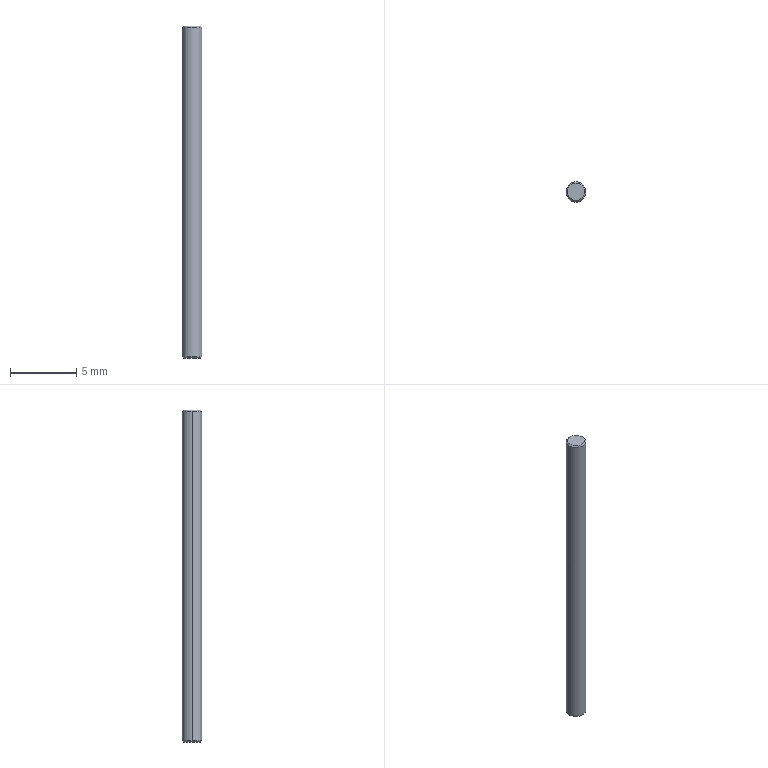Part | SolidWorks | features Chamfer 1, Extrusion 1 | 1 solid | 8 faces | box 1.5 x 1.5 x 25 mm | volume 44.134 mm3 | cone 4 | cylinder 2 | plane 2 | commonest cylinder face diameters 1.5 x2
STEP:
#1=CARTESIAN_POINT('',(0.65,0.,12.5));
#2=VERTEX_POINT('',#1);
#3=CARTESIAN_POINT('',(-0.65,0.,12.5));
#4=VERTEX_POINT('',#3);
#5=CARTESIAN_POINT('',(0.,0.,12.5));
#6=DIRECTION('',(0.,0.,1.));
#7=DIRECTION('',(1.,0.,0.));
#8=AXIS2_PLACEMENT_3D('',#5,#6,#7);
#9=CIRCLE('',#8,0.65);
#10=EDGE_CURVE('',#2,#4,#9,.T.);
#11=ORIENTED_EDGE('',*,*,#10,.F.);
#12=CARTESIAN_POINT('',(0.75,0.,12.4));
#13=VERTEX_POINT('',#12);
#14=CARTESIAN_POINT('',(0.65,0.,12.5));
#15=DIRECTION('',(0.7071,0.,-0.7071));
#16=VECTOR('',#15,1000.);
#17=LINE('',#14,#16);
#18=EDGE_CURVE('',#2,#13,#17,.T.);
#19=ORIENTED_EDGE('',*,*,#18,.T.);
#20=CARTESIAN_POINT('',(-0.75,0.,12.4));
#21=VERTEX_POINT('',#20);
#22=CARTESIAN_POINT('',(0.,0.,12.4));
#23=DIRECTION('',(0.,0.,-1.));
#24=DIRECTION('',(1.,0.,0.));
#25=AXIS2_PLACEMENT_3D('',#22,#23,#24);
#26=CIRCLE('',#25,0.75);
#27=EDGE_CURVE('',#21,#13,#26,.T.);
#28=ORIENTED_EDGE('',*,*,#27,.F.);
#29=CARTESIAN_POINT('',(-0.65,0.,12.5));
#30=DIRECTION('',(-0.7071,0.,-0.7071));
#31=VECTOR('',#30,1000.);
#32=LINE('',#29,#31);
#33=EDGE_CURVE('',#4,#21,#32,.T.);
#34=ORIENTED_EDGE('',*,*,#33,.F.);
#35=EDGE_LOOP('',(#11,#19,#28,#34));
#36=FACE_OUTER_BOUND('',#35,.T.);
#37=CARTESIAN_POINT('',(0.,0.,12.5));
#38=DIRECTION('',(0.,0.,-1.));
#39=DIRECTION('',(-1.,0.,0.));
#40=AXIS2_PLACEMENT_3D('',#37,#38,#39);
#41=CONICAL_SURFACE('',#40,0.65,0.7854);
#42=ADVANCED_FACE('',(#36),#41,.T.);
#43=CARTESIAN_POINT('',(-0.65,0.,-12.5));
#44=VERTEX_POINT('',#43);
#45=CARTESIAN_POINT('',(0.65,0.,-12.5));
#46=VERTEX_POINT('',#45);
#47=CARTESIAN_POINT('',(0.,0.,-12.5));
#48=DIRECTION('',(0.,0.,-1.));
#49=DIRECTION('',(1.,0.,0.));
#50=AXIS2_PLACEMENT_3D('',#47,#48,#49);
#51=CIRCLE('',#50,0.65);
#52=EDGE_CURVE('',#44,#46,#51,.T.);
#53=ORIENTED_EDGE('',*,*,#52,.F.);
#54=CARTESIAN_POINT('',(-0.75,0.,-12.4));
#55=VERTEX_POINT('',#54);
#56=CARTESIAN_POINT('',(-0.75,0.,-12.4));
#57=DIRECTION('',(-0.7071,0.,0.7071));
#58=VECTOR('',#57,1000.);
#59=LINE('',#56,#58);
#60=EDGE_CURVE('',#44,#55,#59,.T.);
#61=ORIENTED_EDGE('',*,*,#60,.T.);
#62=CARTESIAN_POINT('',(0.75,0.,-12.4));
#63=VERTEX_POINT('',#62);
#64=CARTESIAN_POINT('',(0.,0.,-12.4));
#65=DIRECTION('',(0.,0.,1.));
#66=DIRECTION('',(1.,0.,0.));
#67=AXIS2_PLACEMENT_3D('',#64,#65,#66);
#68=CIRCLE('',#67,0.75);
#69=EDGE_CURVE('',#63,#55,#68,.T.);
#70=ORIENTED_EDGE('',*,*,#69,.F.);
#71=CARTESIAN_POINT('',(0.75,0.,-12.4));
#72=DIRECTION('',(0.7071,0.,0.7071));
#73=VECTOR('',#72,1000.);
#74=LINE('',#71,#73);
#75=EDGE_CURVE('',#46,#63,#74,.T.);
#76=ORIENTED_EDGE('',*,*,#75,.F.);
#77=EDGE_LOOP('',(#53,#61,#70,#76));
#78=FACE_OUTER_BOUND('',#77,.T.);
#79=CARTESIAN_POINT('',(0.,0.,-12.4));
#80=DIRECTION('',(0.,0.,1.));
#81=DIRECTION('',(1.,0.,0.));
#82=AXIS2_PLACEMENT_3D('',#79,#80,#81);
#83=CONICAL_SURFACE('',#82,0.75,0.7854);
#84=ADVANCED_FACE('',(#78),#83,.T.);
#85=ORIENTED_EDGE('',*,*,#27,.T.);
#86=CARTESIAN_POINT('',(0.75,0.,12.5));
#87=DIRECTION('',(0.,0.,-1.));
#88=VECTOR('',#87,1000.);
#89=LINE('',#86,#88);
#90=EDGE_CURVE('',#13,#63,#89,.T.);
#91=ORIENTED_EDGE('',*,*,#90,.T.);
#92=ORIENTED_EDGE('',*,*,#69,.T.);
#93=CARTESIAN_POINT('',(-0.75,0.,12.5));
#94=DIRECTION('',(0.,0.,-1.));
#95=VECTOR('',#94,1000.);
#96=LINE('',#93,#95);
#97=EDGE_CURVE('',#21,#55,#96,.T.);
#98=ORIENTED_EDGE('',*,*,#97,.F.);
#99=EDGE_LOOP('',(#85,#91,#92,#98));
#100=FACE_OUTER_BOUND('',#99,.T.);
#101=CARTESIAN_POINT('',(0.,0.,12.5));
#102=DIRECTION('',(0.,0.,-1.));
#103=DIRECTION('',(-1.,0.,0.));
#104=AXIS2_PLACEMENT_3D('',#101,#102,#103);
#105=CYLINDRICAL_SURFACE('',#104,0.75);
#106=ADVANCED_FACE('',(#100),#105,.T.);
#107=ORIENTED_EDGE('',*,*,#90,.F.);
#108=CARTESIAN_POINT('',(0.,0.,12.4));
#109=DIRECTION('',(0.,0.,-1.));
#110=DIRECTION('',(1.,0.,0.));
#111=AXIS2_PLACEMENT_3D('',#108,#109,#110);
#112=CIRCLE('',#111,0.75);
#113=EDGE_CURVE('',#13,#21,#112,.T.);
#114=ORIENTED_EDGE('',*,*,#113,.T.);
#115=ORIENTED_EDGE('',*,*,#97,.T.);
#116=CARTESIAN_POINT('',(0.,0.,-12.4));
#117=DIRECTION('',(0.,0.,1.));
#118=DIRECTION('',(1.,0.,0.));
#119=AXIS2_PLACEMENT_3D('',#116,#117,#118);
#120=CIRCLE('',#119,0.75);
#121=EDGE_CURVE('',#55,#63,#120,.T.);
#122=ORIENTED_EDGE('',*,*,#121,.T.);
#123=EDGE_LOOP('',(#107,#114,#115,#122));
#124=FACE_OUTER_BOUND('',#123,.T.);
#125=CARTESIAN_POINT('',(0.,0.,12.5));
#126=DIRECTION('',(0.,0.,-1.));
#127=DIRECTION('',(-1.,0.,0.));
#128=AXIS2_PLACEMENT_3D('',#125,#126,#127);
#129=CYLINDRICAL_SURFACE('',#128,0.75);
#130=ADVANCED_FACE('',(#124),#129,.T.);
#131=CARTESIAN_POINT('',(0.,0.,12.5));
#132=DIRECTION('',(0.,0.,1.));
#133=DIRECTION('',(1.,0.,0.));
#134=AXIS2_PLACEMENT_3D('',#131,#132,#133);
#135=CIRCLE('',#134,0.65);
#136=EDGE_CURVE('',#4,#2,#135,.T.);
#137=ORIENTED_EDGE('',*,*,#136,.T.);
#138=ORIENTED_EDGE('',*,*,#10,.T.);
#139=EDGE_LOOP('',(#137,#138));
#140=FACE_OUTER_BOUND('',#139,.T.);
#141=CARTESIAN_POINT('',(0.,0.,12.5));
#142=DIRECTION('',(0.,0.,1.));
#143=DIRECTION('',(1.,0.,0.));
#144=AXIS2_PLACEMENT_3D('',#141,#142,#143);
#145=PLANE('',#144);
#146=ADVANCED_FACE('',(#140),#145,.T.);
#147=CARTESIAN_POINT('',(0.,0.,-12.5));
#148=DIRECTION('',(0.,0.,-1.));
#149=DIRECTION('',(1.,0.,0.));
#150=AXIS2_PLACEMENT_3D('',#147,#148,#149);
#151=CIRCLE('',#150,0.65);
#152=EDGE_CURVE('',#46,#44,#151,.T.);
#153=ORIENTED_EDGE('',*,*,#152,.T.);
#154=ORIENTED_EDGE('',*,*,#52,.T.);
#155=EDGE_LOOP('',(#153,#154));
#156=FACE_OUTER_BOUND('',#155,.T.);
#157=CARTESIAN_POINT('',(0.,0.,-12.5));
#158=DIRECTION('',(0.,0.,1.));
#159=DIRECTION('',(1.,0.,0.));
#160=AXIS2_PLACEMENT_3D('',#157,#158,#159);
#161=PLANE('',#160);
#162=ADVANCED_FACE('',(#156),#161,.F.);
#163=ORIENTED_EDGE('',*,*,#60,.F.);
#164=ORIENTED_EDGE('',*,*,#152,.F.);
#165=ORIENTED_EDGE('',*,*,#75,.T.);
#166=ORIENTED_EDGE('',*,*,#121,.F.);
#167=EDGE_LOOP('',(#163,#164,#165,#166));
#168=FACE_OUTER_BOUND('',#167,.T.);
#169=CARTESIAN_POINT('',(0.,0.,-12.4));
#170=DIRECTION('',(0.,0.,1.));
#171=DIRECTION('',(1.,0.,0.));
#172=AXIS2_PLACEMENT_3D('',#169,#170,#171);
#173=CONICAL_SURFACE('',#172,0.75,0.7854);
#174=ADVANCED_FACE('',(#168),#173,.T.);
#175=ORIENTED_EDGE('',*,*,#18,.F.);
#176=ORIENTED_EDGE('',*,*,#136,.F.);
#177=ORIENTED_EDGE('',*,*,#33,.T.);
#178=ORIENTED_EDGE('',*,*,#113,.F.);
#179=EDGE_LOOP('',(#175,#176,#177,#178));
#180=FACE_OUTER_BOUND('',#179,.T.);
#181=CARTESIAN_POINT('',(0.,0.,12.5));
#182=DIRECTION('',(0.,0.,-1.));
#183=DIRECTION('',(-1.,0.,0.));
#184=AXIS2_PLACEMENT_3D('',#181,#182,#183);
#185=CONICAL_SURFACE('',#184,0.65,0.7854);
#186=ADVANCED_FACE('',(#180),#185,.T.);
#187=CLOSED_SHELL('',(#42,#84,#106,#130,#146,#162,#174,#186));
#188=MANIFOLD_SOLID_BREP('',#187);
#189=CARTESIAN_POINT('',(0.,0.,0.));
#190=DIRECTION('',(0.,0.,1.));
#191=DIRECTION('',(1.,0.,0.));
#192=AXIS2_PLACEMENT_3D('',#189,#190,#191);
#193=(LENGTH_UNIT()NAMED_UNIT(*)SI_UNIT(.MILLI.,.METRE.));
#194=UNCERTAINTY_MEASURE_WITH_UNIT(LENGTH_MEASURE(0.00001),#193,'','');
#195=(NAMED_UNIT(*)PLANE_ANGLE_UNIT()SI_UNIT($,.RADIAN.));
#196=(NAMED_UNIT(*)SI_UNIT($,.STERADIAN.)SOLID_ANGLE_UNIT());
#197=(GEOMETRIC_REPRESENTATION_CONTEXT(3)GLOBAL_UNCERTAINTY_ASSIGNED_CONTEXT((#194))GLOBAL_UNIT_ASSIGNED_CONTEXT((#193,#195,#196))REPRESENTATION_CONTEXT('',''));
#198=ADVANCED_BREP_SHAPE_REPRESENTATION('',(#188,#192),#197);